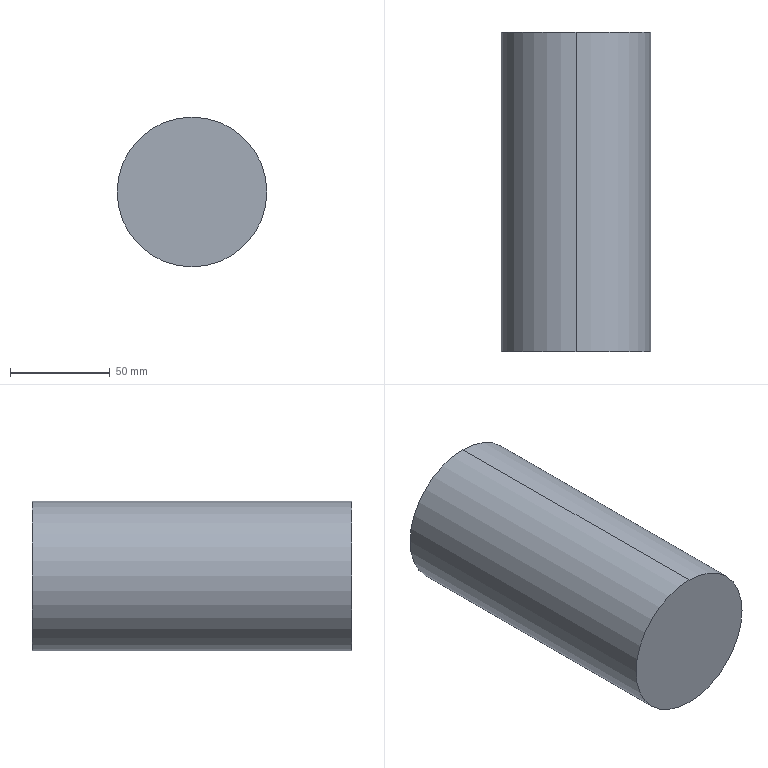Part | SolidWorks | features BaseBody 1 | 1 solid | 4 faces | box 75 x 160 x 75 mm | volume 706858 mm3 | cylinder 2 | plane 2 | commonest cylinder face diameters 75 x2
STEP:
#1=CARTESIAN_POINT('',(0.,160.,-37.5));
#2=VERTEX_POINT('',#1);
#3=CARTESIAN_POINT('',(0.,160.,37.5));
#4=VERTEX_POINT('',#3);
#5=CARTESIAN_POINT('',(0.,160.,0.));
#6=DIRECTION('',(0.,-1.,0.));
#7=DIRECTION('',(0.,0.,-1.));
#8=AXIS2_PLACEMENT_3D('',#5,#6,#7);
#9=CIRCLE('',#8,37.5);
#10=EDGE_CURVE('',#2,#4,#9,.T.);
#11=ORIENTED_EDGE('',*,*,#10,.T.);
#12=CARTESIAN_POINT('',(0.,0.,37.5));
#13=VERTEX_POINT('',#12);
#14=CARTESIAN_POINT('',(0.,160.,37.5));
#15=DIRECTION('',(0.,-1.,0.));
#16=VECTOR('',#15,1000.);
#17=LINE('',#14,#16);
#18=EDGE_CURVE('',#4,#13,#17,.T.);
#19=ORIENTED_EDGE('',*,*,#18,.T.);
#20=CARTESIAN_POINT('',(0.,0.,-37.5));
#21=VERTEX_POINT('',#20);
#22=CARTESIAN_POINT('',(0.,0.,0.));
#23=DIRECTION('',(0.,1.,0.));
#24=DIRECTION('',(0.,0.,-1.));
#25=AXIS2_PLACEMENT_3D('',#22,#23,#24);
#26=CIRCLE('',#25,37.5);
#27=EDGE_CURVE('',#13,#21,#26,.T.);
#28=ORIENTED_EDGE('',*,*,#27,.T.);
#29=CARTESIAN_POINT('',(0.,160.,-37.5));
#30=DIRECTION('',(0.,-1.,0.));
#31=VECTOR('',#30,1000.);
#32=LINE('',#29,#31);
#33=EDGE_CURVE('',#2,#21,#32,.T.);
#34=ORIENTED_EDGE('',*,*,#33,.F.);
#35=EDGE_LOOP('',(#11,#19,#28,#34));
#36=FACE_OUTER_BOUND('',#35,.T.);
#37=CARTESIAN_POINT('',(0.,160.,0.));
#38=DIRECTION('',(0.,-1.,0.));
#39=DIRECTION('',(0.,0.,-1.));
#40=AXIS2_PLACEMENT_3D('',#37,#38,#39);
#41=CYLINDRICAL_SURFACE('',#40,37.5);
#42=ADVANCED_FACE('',(#36),#41,.T.);
#43=ORIENTED_EDGE('',*,*,#18,.F.);
#44=CARTESIAN_POINT('',(0.,160.,0.));
#45=DIRECTION('',(0.,-1.,0.));
#46=DIRECTION('',(0.,0.,-1.));
#47=AXIS2_PLACEMENT_3D('',#44,#45,#46);
#48=CIRCLE('',#47,37.5);
#49=EDGE_CURVE('',#4,#2,#48,.T.);
#50=ORIENTED_EDGE('',*,*,#49,.T.);
#51=ORIENTED_EDGE('',*,*,#33,.T.);
#52=CARTESIAN_POINT('',(0.,0.,0.));
#53=DIRECTION('',(0.,1.,0.));
#54=DIRECTION('',(0.,0.,-1.));
#55=AXIS2_PLACEMENT_3D('',#52,#53,#54);
#56=CIRCLE('',#55,37.5);
#57=EDGE_CURVE('',#21,#13,#56,.T.);
#58=ORIENTED_EDGE('',*,*,#57,.T.);
#59=EDGE_LOOP('',(#43,#50,#51,#58));
#60=FACE_OUTER_BOUND('',#59,.T.);
#61=CARTESIAN_POINT('',(0.,160.,0.));
#62=DIRECTION('',(0.,-1.,0.));
#63=DIRECTION('',(0.,0.,-1.));
#64=AXIS2_PLACEMENT_3D('',#61,#62,#63);
#65=CYLINDRICAL_SURFACE('',#64,37.5);
#66=ADVANCED_FACE('',(#60),#65,.T.);
#67=ORIENTED_EDGE('',*,*,#57,.F.);
#68=ORIENTED_EDGE('',*,*,#27,.F.);
#69=EDGE_LOOP('',(#67,#68));
#70=FACE_OUTER_BOUND('',#69,.T.);
#71=CARTESIAN_POINT('',(0.,0.,0.));
#72=DIRECTION('',(0.,1.,0.));
#73=DIRECTION('',(0.,0.,1.));
#74=AXIS2_PLACEMENT_3D('',#71,#72,#73);
#75=PLANE('',#74);
#76=ADVANCED_FACE('',(#70),#75,.F.);
#77=ORIENTED_EDGE('',*,*,#10,.F.);
#78=ORIENTED_EDGE('',*,*,#49,.F.);
#79=EDGE_LOOP('',(#77,#78));
#80=FACE_OUTER_BOUND('',#79,.T.);
#81=CARTESIAN_POINT('',(0.,160.,0.));
#82=DIRECTION('',(0.,1.,0.));
#83=DIRECTION('',(0.,0.,1.));
#84=AXIS2_PLACEMENT_3D('',#81,#82,#83);
#85=PLANE('',#84);
#86=ADVANCED_FACE('',(#80),#85,.T.);
#87=CLOSED_SHELL('',(#42,#66,#76,#86));
#88=MANIFOLD_SOLID_BREP('',#87);
#89=CARTESIAN_POINT('',(0.,0.,0.));
#90=DIRECTION('',(0.,0.,1.));
#91=DIRECTION('',(1.,0.,0.));
#92=AXIS2_PLACEMENT_3D('',#89,#90,#91);
#93=(LENGTH_UNIT()NAMED_UNIT(*)SI_UNIT(.MILLI.,.METRE.));
#94=UNCERTAINTY_MEASURE_WITH_UNIT(LENGTH_MEASURE(0.00001),#93,'','');
#95=(NAMED_UNIT(*)PLANE_ANGLE_UNIT()SI_UNIT($,.RADIAN.));
#96=(NAMED_UNIT(*)SI_UNIT($,.STERADIAN.)SOLID_ANGLE_UNIT());
#97=(GEOMETRIC_REPRESENTATION_CONTEXT(3)GLOBAL_UNCERTAINTY_ASSIGNED_CONTEXT((#94))GLOBAL_UNIT_ASSIGNED_CONTEXT((#93,#95,#96))REPRESENTATION_CONTEXT('',''));
#98=ADVANCED_BREP_SHAPE_REPRESENTATION('',(#88,#92),#97);